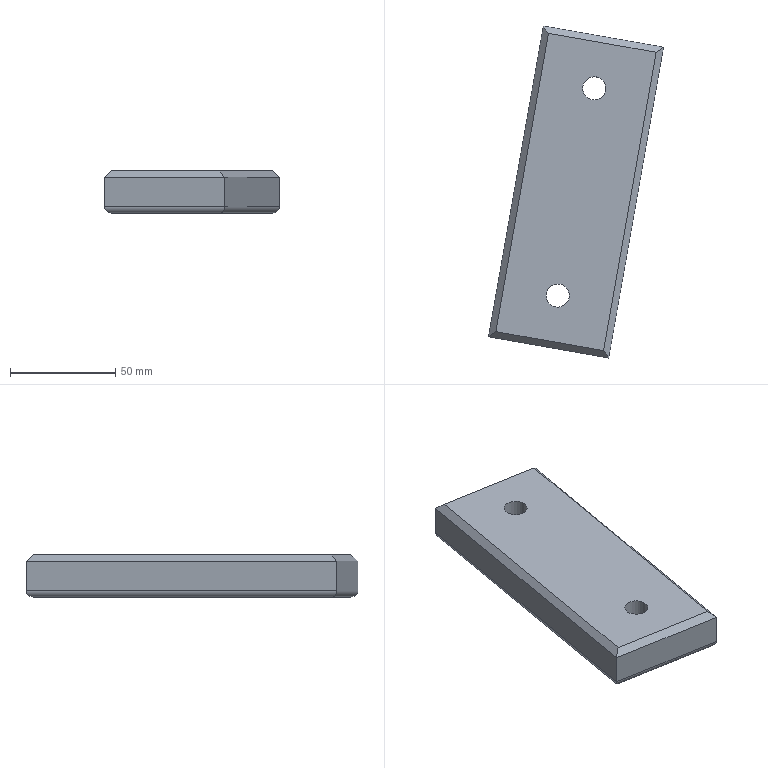Part | NX | features solid 2 | 1 solid | 20 faces | box 83.166 x 157.793 x 20 mm | volume 164078 mm3 | plane 12 | cylinder 8 | commonest cylinder face diameters 6 x4 11 x2 17.5 x2
STEP:
#1=CARTESIAN_POINT('',(863.455,-228.407,187.));
#2=VERTEX_POINT('',#1);
#3=CARTESIAN_POINT('',(863.455,-228.407,173.));
#4=VERTEX_POINT('',#3);
#5=CARTESIAN_POINT('',(863.455,-228.407,190.));
#6=DIRECTION('',(0.,0.,-1.));
#7=VECTOR('',#6,1000.);
#8=LINE('',#5,#7);
#9=EDGE_CURVE('',#2,#4,#8,.T.);
#10=ORIENTED_EDGE('',*,*,#9,.F.);
#11=CARTESIAN_POINT('',(806.336,-218.336,187.));
#12=VERTEX_POINT('',#11);
#13=CARTESIAN_POINT('',(806.336,-218.336,187.));
#14=DIRECTION('',(-0.9848,0.1736,0.));
#15=VECTOR('',#14,1000.);
#16=LINE('',#13,#15);
#17=EDGE_CURVE('',#2,#12,#16,.T.);
#18=ORIENTED_EDGE('',*,*,#17,.T.);
#19=CARTESIAN_POINT('',(806.336,-218.336,173.));
#20=VERTEX_POINT('',#19);
#21=CARTESIAN_POINT('',(806.336,-218.336,190.));
#22=DIRECTION('',(0.,0.,-1.));
#23=VECTOR('',#22,1000.);
#24=LINE('',#21,#23);
#25=EDGE_CURVE('',#12,#20,#24,.T.);
#26=ORIENTED_EDGE('',*,*,#25,.T.);
#27=CARTESIAN_POINT('',(806.336,-218.336,173.));
#28=DIRECTION('',(0.9848,-0.1736,0.));
#29=VECTOR('',#28,1000.);
#30=LINE('',#27,#29);
#31=EDGE_CURVE('',#20,#4,#30,.T.);
#32=ORIENTED_EDGE('',*,*,#31,.T.);
#33=EDGE_LOOP('',(#10,#18,#26,#32));
#34=FACE_BOUND('',#33,.T.);
#35=CARTESIAN_POINT('',(806.336,-218.336,190.));
#36=DIRECTION('',(0.1736,0.9848,0.));
#37=DIRECTION('',(0.,0.,-1.));
#38=AXIS2_PLACEMENT_3D('',#35,#36,#37);
#39=PLANE('',#38);
#40=ADVANCED_FACE('',(#34),#39,.F.);
#41=CARTESIAN_POINT('',(889.503,-80.686,187.));
#42=VERTEX_POINT('',#41);
#43=CARTESIAN_POINT('',(889.503,-80.686,173.));
#44=VERTEX_POINT('',#43);
#45=CARTESIAN_POINT('',(889.503,-80.686,190.));
#46=DIRECTION('',(0.,0.,-1.));
#47=VECTOR('',#46,1000.);
#48=LINE('',#45,#47);
#49=EDGE_CURVE('',#42,#44,#48,.T.);
#50=ORIENTED_EDGE('',*,*,#49,.F.);
#51=CARTESIAN_POINT('',(863.455,-228.407,187.));
#52=DIRECTION('',(-0.1736,-0.9848,0.));
#53=VECTOR('',#52,1000.);
#54=LINE('',#51,#53);
#55=EDGE_CURVE('',#42,#2,#54,.T.);
#56=ORIENTED_EDGE('',*,*,#55,.T.);
#57=ORIENTED_EDGE('',*,*,#9,.T.);
#58=CARTESIAN_POINT('',(863.455,-228.407,173.));
#59=DIRECTION('',(0.1736,0.9848,0.));
#60=VECTOR('',#59,1000.);
#61=LINE('',#58,#60);
#62=EDGE_CURVE('',#4,#44,#61,.T.);
#63=ORIENTED_EDGE('',*,*,#62,.T.);
#64=EDGE_LOOP('',(#50,#56,#57,#63));
#65=FACE_BOUND('',#64,.T.);
#66=CARTESIAN_POINT('',(863.455,-228.407,190.));
#67=DIRECTION('',(-0.9848,0.1736,0.));
#68=DIRECTION('',(0.,0.,1.));
#69=AXIS2_PLACEMENT_3D('',#66,#67,#68);
#70=PLANE('',#69);
#71=ADVANCED_FACE('',(#65),#70,.F.);
#72=CARTESIAN_POINT('',(832.384,-70.615,187.));
#73=VERTEX_POINT('',#72);
#74=CARTESIAN_POINT('',(832.384,-70.615,173.));
#75=VERTEX_POINT('',#74);
#76=CARTESIAN_POINT('',(832.384,-70.615,190.));
#77=DIRECTION('',(0.,0.,-1.));
#78=VECTOR('',#77,1000.);
#79=LINE('',#76,#78);
#80=EDGE_CURVE('',#73,#75,#79,.T.);
#81=ORIENTED_EDGE('',*,*,#80,.F.);
#82=CARTESIAN_POINT('',(889.503,-80.686,187.));
#83=DIRECTION('',(0.9848,-0.1736,0.));
#84=VECTOR('',#83,1000.);
#85=LINE('',#82,#84);
#86=EDGE_CURVE('',#73,#42,#85,.T.);
#87=ORIENTED_EDGE('',*,*,#86,.T.);
#88=ORIENTED_EDGE('',*,*,#49,.T.);
#89=CARTESIAN_POINT('',(889.503,-80.686,173.));
#90=DIRECTION('',(-0.9848,0.1736,0.));
#91=VECTOR('',#90,1000.);
#92=LINE('',#89,#91);
#93=EDGE_CURVE('',#44,#75,#92,.T.);
#94=ORIENTED_EDGE('',*,*,#93,.T.);
#95=EDGE_LOOP('',(#81,#87,#88,#94));
#96=FACE_BOUND('',#95,.T.);
#97=CARTESIAN_POINT('',(889.503,-80.686,190.));
#98=DIRECTION('',(-0.1736,-0.9848,0.));
#99=DIRECTION('',(0.,0.,1.));
#100=AXIS2_PLACEMENT_3D('',#97,#98,#99);
#101=PLANE('',#100);
#102=ADVANCED_FACE('',(#96),#101,.F.);
#103=ORIENTED_EDGE('',*,*,#25,.F.);
#104=CARTESIAN_POINT('',(832.384,-70.615,187.));
#105=DIRECTION('',(0.1736,0.9848,0.));
#106=VECTOR('',#105,1000.);
#107=LINE('',#104,#106);
#108=EDGE_CURVE('',#12,#73,#107,.T.);
#109=ORIENTED_EDGE('',*,*,#108,.T.);
#110=ORIENTED_EDGE('',*,*,#80,.T.);
#111=CARTESIAN_POINT('',(832.384,-70.615,173.));
#112=DIRECTION('',(-0.1736,-0.9848,0.));
#113=VECTOR('',#112,1000.);
#114=LINE('',#111,#113);
#115=EDGE_CURVE('',#75,#20,#114,.T.);
#116=ORIENTED_EDGE('',*,*,#115,.T.);
#117=EDGE_LOOP('',(#103,#109,#110,#116));
#118=FACE_BOUND('',#117,.T.);
#119=CARTESIAN_POINT('',(832.384,-70.615,190.));
#120=DIRECTION('',(0.9848,-0.1736,0.));
#121=DIRECTION('',(0.1736,0.9848,0.));
#122=AXIS2_PLACEMENT_3D('',#119,#120,#121);
#123=PLANE('',#122);
#124=ADVANCED_FACE('',(#118),#123,.F.);
#125=CARTESIAN_POINT('',(861.022,-224.932,190.));
#126=VERTEX_POINT('',#125);
#127=CARTESIAN_POINT('',(886.027,-83.12,190.));
#128=VERTEX_POINT('',#127);
#129=CARTESIAN_POINT('',(886.548,-80.165,190.));
#130=DIRECTION('',(0.1736,0.9848,0.));
#131=VECTOR('',#130,1000.);
#132=LINE('',#129,#131);
#133=EDGE_CURVE('',#126,#128,#132,.T.);
#134=ORIENTED_EDGE('',*,*,#133,.T.);
#135=CARTESIAN_POINT('',(834.817,-74.09,190.));
#136=VERTEX_POINT('',#135);
#137=CARTESIAN_POINT('',(831.863,-73.569,190.));
#138=DIRECTION('',(-0.9848,0.1736,0.));
#139=VECTOR('',#138,1000.);
#140=LINE('',#137,#139);
#141=EDGE_CURVE('',#128,#136,#140,.T.);
#142=ORIENTED_EDGE('',*,*,#141,.T.);
#143=CARTESIAN_POINT('',(809.812,-215.902,190.));
#144=VERTEX_POINT('',#143);
#145=CARTESIAN_POINT('',(809.291,-218.857,190.));
#146=DIRECTION('',(-0.1736,-0.9848,0.));
#147=VECTOR('',#146,1000.);
#148=LINE('',#145,#147);
#149=EDGE_CURVE('',#136,#144,#148,.T.);
#150=ORIENTED_EDGE('',*,*,#149,.T.);
#151=CARTESIAN_POINT('',(863.976,-225.453,190.));
#152=DIRECTION('',(0.9848,-0.1736,0.));
#153=VECTOR('',#152,1000.);
#154=LINE('',#151,#153);
#155=EDGE_CURVE('',#144,#126,#154,.T.);
#156=ORIENTED_EDGE('',*,*,#155,.T.);
#157=EDGE_LOOP('',(#134,#142,#150,#156));
#158=FACE_BOUND('',#157,.T.);
#159=CARTESIAN_POINT('',(857.557,-94.854,190.));
#160=VERTEX_POINT('',#159);
#161=CARTESIAN_POINT('',(856.602,-100.271,190.));
#162=DIRECTION('',(0.,0.,1.));
#163=DIRECTION('',(0.1736,0.9848,0.));
#164=AXIS2_PLACEMENT_3D('',#161,#162,#163);
#165=CIRCLE('',#164,5.5);
#166=EDGE_CURVE('',#160,#160,#165,.T.);
#167=ORIENTED_EDGE('',*,*,#166,.F.);
#168=EDGE_LOOP('',(#167));
#169=FACE_BOUND('',#168,.T.);
#170=CARTESIAN_POINT('',(840.192,-193.335,190.));
#171=VERTEX_POINT('',#170);
#172=CARTESIAN_POINT('',(839.237,-198.751,190.));
#173=DIRECTION('',(0.,0.,1.));
#174=DIRECTION('',(0.1736,0.9848,0.));
#175=AXIS2_PLACEMENT_3D('',#172,#173,#174);
#176=CIRCLE('',#175,5.5);
#177=EDGE_CURVE('',#171,#171,#176,.T.);
#178=ORIENTED_EDGE('',*,*,#177,.F.);
#179=EDGE_LOOP('',(#178));
#180=FACE_BOUND('',#179,.T.);
#181=CARTESIAN_POINT('',(863.455,-228.407,190.));
#182=DIRECTION('',(0.,0.,1.));
#183=DIRECTION('',(0.1736,0.9848,0.));
#184=AXIS2_PLACEMENT_3D('',#181,#182,#183);
#185=PLANE('',#184);
#186=ADVANCED_FACE('',(#158,#169,#180),#185,.T.);
#187=CARTESIAN_POINT('',(861.022,-224.932,170.));
#188=VERTEX_POINT('',#187);
#189=CARTESIAN_POINT('',(809.812,-215.902,170.));
#190=VERTEX_POINT('',#189);
#191=CARTESIAN_POINT('',(863.976,-225.453,170.));
#192=DIRECTION('',(0.9848,-0.1736,0.));
#193=VECTOR('',#192,1000.);
#194=LINE('',#191,#193);
#195=EDGE_CURVE('',#188,#190,#194,.F.);
#196=ORIENTED_EDGE('',*,*,#195,.T.);
#197=CARTESIAN_POINT('',(834.817,-74.09,170.));
#198=VERTEX_POINT('',#197);
#199=CARTESIAN_POINT('',(809.291,-218.857,170.));
#200=DIRECTION('',(-0.1736,-0.9848,0.));
#201=VECTOR('',#200,1000.);
#202=LINE('',#199,#201);
#203=EDGE_CURVE('',#190,#198,#202,.F.);
#204=ORIENTED_EDGE('',*,*,#203,.T.);
#205=CARTESIAN_POINT('',(886.027,-83.12,170.));
#206=VERTEX_POINT('',#205);
#207=CARTESIAN_POINT('',(888.982,-83.641,170.));
#208=DIRECTION('',(-0.9848,0.1736,0.));
#209=VECTOR('',#208,1000.);
#210=LINE('',#207,#209);
#211=EDGE_CURVE('',#198,#206,#210,.F.);
#212=ORIENTED_EDGE('',*,*,#211,.T.);
#213=CARTESIAN_POINT('',(860.501,-227.887,170.));
#214=DIRECTION('',(0.1736,0.9848,0.));
#215=VECTOR('',#214,1000.);
#216=LINE('',#213,#215);
#217=EDGE_CURVE('',#206,#188,#216,.F.);
#218=ORIENTED_EDGE('',*,*,#217,.T.);
#219=EDGE_LOOP('',(#196,#204,#212,#218));
#220=FACE_BOUND('',#219,.T.);
#221=CARTESIAN_POINT('',(858.121,-91.654,170.));
#222=VERTEX_POINT('',#221);
#223=CARTESIAN_POINT('',(856.602,-100.271,170.));
#224=DIRECTION('',(0.,0.,1.));
#225=DIRECTION('',(0.1736,0.9848,0.));
#226=AXIS2_PLACEMENT_3D('',#223,#224,#225);
#227=CIRCLE('',#226,8.75);
#228=EDGE_CURVE('',#222,#222,#227,.T.);
#229=ORIENTED_EDGE('',*,*,#228,.T.);
#230=EDGE_LOOP('',(#229));
#231=FACE_BOUND('',#230,.T.);
#232=CARTESIAN_POINT('',(840.756,-190.134,170.));
#233=VERTEX_POINT('',#232);
#234=CARTESIAN_POINT('',(839.237,-198.751,170.));
#235=DIRECTION('',(0.,0.,1.));
#236=DIRECTION('',(0.1736,0.9848,0.));
#237=AXIS2_PLACEMENT_3D('',#234,#235,#236);
#238=CIRCLE('',#237,8.75);
#239=EDGE_CURVE('',#233,#233,#238,.T.);
#240=ORIENTED_EDGE('',*,*,#239,.T.);
#241=EDGE_LOOP('',(#240));
#242=FACE_BOUND('',#241,.T.);
#243=CARTESIAN_POINT('',(863.455,-228.407,170.));
#244=DIRECTION('',(0.,0.,1.));
#245=DIRECTION('',(0.1736,0.9848,0.));
#246=AXIS2_PLACEMENT_3D('',#243,#244,#245);
#247=PLANE('',#246);
#248=ADVANCED_FACE('',(#220,#231,#242),#247,.F.);
#249=ORIENTED_EDGE('',*,*,#177,.T.);
#250=EDGE_LOOP('',(#249));
#251=FACE_BOUND('',#250,.T.);
#252=CARTESIAN_POINT('',(840.192,-193.335,182.));
#253=VERTEX_POINT('',#252);
#254=CARTESIAN_POINT('',(839.237,-198.751,182.));
#255=DIRECTION('',(0.,0.,1.));
#256=DIRECTION('',(0.1736,0.9848,0.));
#257=AXIS2_PLACEMENT_3D('',#254,#255,#256);
#258=CIRCLE('',#257,5.5);
#259=EDGE_CURVE('',#253,#253,#258,.T.);
#260=ORIENTED_EDGE('',*,*,#259,.F.);
#261=EDGE_LOOP('',(#260));
#262=FACE_BOUND('',#261,.T.);
#263=CARTESIAN_POINT('',(839.237,-198.751,220.));
#264=DIRECTION('',(0.,0.,1.));
#265=DIRECTION('',(0.1736,0.9848,0.));
#266=AXIS2_PLACEMENT_3D('',#263,#264,#265);
#267=CYLINDRICAL_SURFACE('',#266,5.5);
#268=ADVANCED_FACE('',(#251,#262),#267,.F.);
#269=ORIENTED_EDGE('',*,*,#259,.T.);
#270=EDGE_LOOP('',(#269));
#271=FACE_BOUND('',#270,.T.);
#272=CARTESIAN_POINT('',(840.756,-190.134,182.));
#273=VERTEX_POINT('',#272);
#274=CARTESIAN_POINT('',(839.237,-198.751,182.));
#275=DIRECTION('',(0.,0.,1.));
#276=DIRECTION('',(0.1736,0.9848,0.));
#277=AXIS2_PLACEMENT_3D('',#274,#275,#276);
#278=CIRCLE('',#277,8.75);
#279=EDGE_CURVE('',#273,#273,#278,.T.);
#280=ORIENTED_EDGE('',*,*,#279,.F.);
#281=EDGE_LOOP('',(#280));
#282=FACE_BOUND('',#281,.T.);
#283=CARTESIAN_POINT('',(839.237,-198.751,182.));
#284=DIRECTION('',(0.,0.,1.));
#285=DIRECTION('',(0.1736,0.9848,0.));
#286=AXIS2_PLACEMENT_3D('',#283,#284,#285);
#287=PLANE('',#286);
#288=ADVANCED_FACE('',(#271,#282),#287,.F.);
#289=ORIENTED_EDGE('',*,*,#279,.T.);
#290=EDGE_LOOP('',(#289));
#291=FACE_BOUND('',#290,.T.);
#292=ORIENTED_EDGE('',*,*,#239,.F.);
#293=EDGE_LOOP('',(#292));
#294=FACE_BOUND('',#293,.T.);
#295=CARTESIAN_POINT('',(839.237,-198.751,170.));
#296=DIRECTION('',(0.,0.,1.));
#297=DIRECTION('',(0.1736,0.9848,0.));
#298=AXIS2_PLACEMENT_3D('',#295,#296,#297);
#299=CYLINDRICAL_SURFACE('',#298,8.75);
#300=ADVANCED_FACE('',(#291,#294),#299,.F.);
#301=ORIENTED_EDGE('',*,*,#166,.T.);
#302=EDGE_LOOP('',(#301));
#303=FACE_BOUND('',#302,.T.);
#304=CARTESIAN_POINT('',(857.557,-94.854,182.));
#305=VERTEX_POINT('',#304);
#306=CARTESIAN_POINT('',(856.602,-100.271,182.));
#307=DIRECTION('',(0.,0.,1.));
#308=DIRECTION('',(0.1736,0.9848,0.));
#309=AXIS2_PLACEMENT_3D('',#306,#307,#308);
#310=CIRCLE('',#309,5.5);
#311=EDGE_CURVE('',#305,#305,#310,.T.);
#312=ORIENTED_EDGE('',*,*,#311,.F.);
#313=EDGE_LOOP('',(#312));
#314=FACE_BOUND('',#313,.T.);
#315=CARTESIAN_POINT('',(856.602,-100.271,220.));
#316=DIRECTION('',(0.,0.,1.));
#317=DIRECTION('',(0.1736,0.9848,0.));
#318=AXIS2_PLACEMENT_3D('',#315,#316,#317);
#319=CYLINDRICAL_SURFACE('',#318,5.5);
#320=ADVANCED_FACE('',(#303,#314),#319,.F.);
#321=ORIENTED_EDGE('',*,*,#311,.T.);
#322=EDGE_LOOP('',(#321));
#323=FACE_BOUND('',#322,.T.);
#324=CARTESIAN_POINT('',(858.121,-91.654,182.));
#325=VERTEX_POINT('',#324);
#326=CARTESIAN_POINT('',(856.602,-100.271,182.));
#327=DIRECTION('',(0.,0.,1.));
#328=DIRECTION('',(0.1736,0.9848,0.));
#329=AXIS2_PLACEMENT_3D('',#326,#327,#328);
#330=CIRCLE('',#329,8.75);
#331=EDGE_CURVE('',#325,#325,#330,.T.);
#332=ORIENTED_EDGE('',*,*,#331,.F.);
#333=EDGE_LOOP('',(#332));
#334=FACE_BOUND('',#333,.T.);
#335=CARTESIAN_POINT('',(856.602,-100.271,182.));
#336=DIRECTION('',(0.,0.,1.));
#337=DIRECTION('',(0.1736,0.9848,0.));
#338=AXIS2_PLACEMENT_3D('',#335,#336,#337);
#339=PLANE('',#338);
#340=ADVANCED_FACE('',(#323,#334),#339,.F.);
#341=ORIENTED_EDGE('',*,*,#331,.T.);
#342=EDGE_LOOP('',(#341));
#343=FACE_BOUND('',#342,.T.);
#344=ORIENTED_EDGE('',*,*,#228,.F.);
#345=EDGE_LOOP('',(#344));
#346=FACE_BOUND('',#345,.T.);
#347=CARTESIAN_POINT('',(856.602,-100.271,170.));
#348=DIRECTION('',(0.,0.,1.));
#349=DIRECTION('',(0.1736,0.9848,0.));
#350=AXIS2_PLACEMENT_3D('',#347,#348,#349);
#351=CYLINDRICAL_SURFACE('',#350,8.75);
#352=ADVANCED_FACE('',(#343,#346),#351,.F.);
#353=CARTESIAN_POINT('',(861.022,-224.932,173.));
#354=DIRECTION('',(0.8192,0.5736,0.));
#355=DIRECTION('',(0.5736,-0.8192,0.));
#356=AXIS2_PLACEMENT_3D('',#353,#354,#355);
#357=ELLIPSE('',#356,4.243,3.);
#358=EDGE_CURVE('',#188,#4,#357,.F.);
#359=ORIENTED_EDGE('',*,*,#358,.F.);
#360=ORIENTED_EDGE('',*,*,#217,.F.);
#361=CARTESIAN_POINT('',(886.027,-83.12,173.));
#362=DIRECTION('',(-0.5736,0.8192,0.));
#363=DIRECTION('',(0.8192,0.5736,0.));
#364=AXIS2_PLACEMENT_3D('',#361,#362,#363);
#365=ELLIPSE('',#364,4.243,3.);
#366=EDGE_CURVE('',#44,#206,#365,.T.);
#367=ORIENTED_EDGE('',*,*,#366,.F.);
#368=ORIENTED_EDGE('',*,*,#62,.F.);
#369=EDGE_LOOP('',(#359,#360,#367,#368));
#370=FACE_BOUND('',#369,.T.);
#371=CARTESIAN_POINT('',(860.501,-227.887,173.));
#372=DIRECTION('',(0.1736,0.9848,0.));
#373=DIRECTION('',(0.,0.,-1.));
#374=AXIS2_PLACEMENT_3D('',#371,#372,#373);
#375=CYLINDRICAL_SURFACE('',#374,3.);
#376=ADVANCED_FACE('',(#370),#375,.T.);
#377=ORIENTED_EDGE('',*,*,#366,.T.);
#378=ORIENTED_EDGE('',*,*,#211,.F.);
#379=CARTESIAN_POINT('',(834.817,-74.09,173.));
#380=DIRECTION('',(-0.8192,-0.5736,0.));
#381=DIRECTION('',(-0.5736,0.8192,0.));
#382=AXIS2_PLACEMENT_3D('',#379,#380,#381);
#383=ELLIPSE('',#382,4.243,3.);
#384=EDGE_CURVE('',#75,#198,#383,.T.);
#385=ORIENTED_EDGE('',*,*,#384,.F.);
#386=ORIENTED_EDGE('',*,*,#93,.F.);
#387=EDGE_LOOP('',(#377,#378,#385,#386));
#388=FACE_BOUND('',#387,.T.);
#389=CARTESIAN_POINT('',(888.982,-83.641,173.));
#390=DIRECTION('',(-0.9848,0.1736,0.));
#391=DIRECTION('',(0.,0.,1.));
#392=AXIS2_PLACEMENT_3D('',#389,#390,#391);
#393=CYLINDRICAL_SURFACE('',#392,3.);
#394=ADVANCED_FACE('',(#388),#393,.T.);
#395=ORIENTED_EDGE('',*,*,#358,.T.);
#396=ORIENTED_EDGE('',*,*,#31,.F.);
#397=CARTESIAN_POINT('',(809.812,-215.902,173.));
#398=DIRECTION('',(0.5736,-0.8192,0.));
#399=DIRECTION('',(0.8192,0.5736,0.));
#400=AXIS2_PLACEMENT_3D('',#397,#398,#399);
#401=ELLIPSE('',#400,4.243,3.);
#402=EDGE_CURVE('',#190,#20,#401,.F.);
#403=ORIENTED_EDGE('',*,*,#402,.F.);
#404=ORIENTED_EDGE('',*,*,#195,.F.);
#405=EDGE_LOOP('',(#395,#396,#403,#404));
#406=FACE_BOUND('',#405,.T.);
#407=CARTESIAN_POINT('',(806.857,-215.381,173.));
#408=DIRECTION('',(0.9848,-0.1736,0.));
#409=DIRECTION('',(0.,0.,-1.));
#410=AXIS2_PLACEMENT_3D('',#407,#408,#409);
#411=CYLINDRICAL_SURFACE('',#410,3.);
#412=ADVANCED_FACE('',(#406),#411,.T.);
#413=ORIENTED_EDGE('',*,*,#384,.T.);
#414=ORIENTED_EDGE('',*,*,#203,.F.);
#415=ORIENTED_EDGE('',*,*,#402,.T.);
#416=ORIENTED_EDGE('',*,*,#115,.F.);
#417=EDGE_LOOP('',(#413,#414,#415,#416));
#418=FACE_BOUND('',#417,.T.);
#419=CARTESIAN_POINT('',(835.338,-71.136,173.));
#420=DIRECTION('',(-0.1736,-0.9848,0.));
#421=DIRECTION('',(0.9848,-0.1736,0.));
#422=AXIS2_PLACEMENT_3D('',#419,#420,#421);
#423=CYLINDRICAL_SURFACE('',#422,3.);
#424=ADVANCED_FACE('',(#418),#423,.T.);
#425=CARTESIAN_POINT('',(808.653,-216.714,189.));
#426=DIRECTION('',(0.6688,0.4683,0.5774));
#427=VECTOR('',#426,1000.);
#428=LINE('',#425,#427);
#429=EDGE_CURVE('',#12,#144,#428,.T.);
#430=ORIENTED_EDGE('',*,*,#429,.F.);
#431=ORIENTED_EDGE('',*,*,#17,.F.);
#432=CARTESIAN_POINT('',(861.833,-226.091,189.));
#433=DIRECTION('',(-0.4683,0.6688,0.5774));
#434=VECTOR('',#433,1000.);
#435=LINE('',#432,#434);
#436=EDGE_CURVE('',#126,#2,#435,.F.);
#437=ORIENTED_EDGE('',*,*,#436,.F.);
#438=ORIENTED_EDGE('',*,*,#155,.F.);
#439=EDGE_LOOP('',(#430,#431,#437,#438));
#440=FACE_BOUND('',#439,.T.);
#441=CARTESIAN_POINT('',(863.976,-225.453,190.));
#442=DIRECTION('',(-0.1228,-0.6964,0.7071));
#443=DIRECTION('',(0.1228,0.6964,0.7071));
#444=AXIS2_PLACEMENT_3D('',#441,#442,#443);
#445=PLANE('',#444);
#446=ADVANCED_FACE('',(#440),#445,.T.);
#447=ORIENTED_EDGE('',*,*,#436,.T.);
#448=ORIENTED_EDGE('',*,*,#55,.F.);
#449=CARTESIAN_POINT('',(829.263,-122.867,239.));
#450=DIRECTION('',(-0.6688,-0.4683,0.5774));
#451=VECTOR('',#450,1000.);
#452=LINE('',#449,#451);
#453=EDGE_CURVE('',#128,#42,#452,.F.);
#454=ORIENTED_EDGE('',*,*,#453,.F.);
#455=ORIENTED_EDGE('',*,*,#133,.F.);
#456=EDGE_LOOP('',(#447,#448,#454,#455));
#457=FACE_BOUND('',#456,.T.);
#458=CARTESIAN_POINT('',(860.501,-227.887,190.));
#459=DIRECTION('',(0.6964,-0.1228,0.7071));
#460=DIRECTION('',(0.6964,-0.1228,-0.7071));
#461=AXIS2_PLACEMENT_3D('',#458,#459,#460);
#462=PLANE('',#461);
#463=ADVANCED_FACE('',(#457),#462,.T.);
#464=ORIENTED_EDGE('',*,*,#429,.T.);
#465=ORIENTED_EDGE('',*,*,#149,.F.);
#466=CARTESIAN_POINT('',(874.564,-130.854,239.));
#467=DIRECTION('',(-0.4683,0.6688,-0.5774));
#468=VECTOR('',#467,1000.);
#469=LINE('',#466,#468);
#470=EDGE_CURVE('',#73,#136,#469,.F.);
#471=ORIENTED_EDGE('',*,*,#470,.F.);
#472=ORIENTED_EDGE('',*,*,#108,.F.);
#473=EDGE_LOOP('',(#464,#465,#471,#472));
#474=FACE_BOUND('',#473,.T.);
#475=CARTESIAN_POINT('',(809.291,-218.857,190.));
#476=DIRECTION('',(-0.6964,0.1228,0.7071));
#477=DIRECTION('',(0.6964,-0.1228,0.7071));
#478=AXIS2_PLACEMENT_3D('',#475,#476,#477);
#479=PLANE('',#478);
#480=ADVANCED_FACE('',(#474),#479,.T.);
#481=ORIENTED_EDGE('',*,*,#453,.T.);
#482=ORIENTED_EDGE('',*,*,#86,.F.);
#483=ORIENTED_EDGE('',*,*,#470,.T.);
#484=ORIENTED_EDGE('',*,*,#141,.F.);
#485=EDGE_LOOP('',(#481,#482,#483,#484));
#486=FACE_BOUND('',#485,.T.);
#487=CARTESIAN_POINT('',(888.982,-83.641,190.));
#488=DIRECTION('',(0.1228,0.6964,0.7071));
#489=DIRECTION('',(0.1228,0.6964,-0.7071));
#490=AXIS2_PLACEMENT_3D('',#487,#488,#489);
#491=PLANE('',#490);
#492=ADVANCED_FACE('',(#486),#491,.T.);
#493=CLOSED_SHELL('',(#40,#71,#102,#124,#186,#248,#268,#288,#300,#320,#340,#352,#376,#394,#412,#424,#446,#463,#480,#492));
#494=MANIFOLD_SOLID_BREP('',#493);
#495=(LENGTH_UNIT()NAMED_UNIT(*)SI_UNIT(.MILLI.,.METRE.));
#496=UNCERTAINTY_MEASURE_WITH_UNIT(LENGTH_MEASURE(0.00001),#495,'','');
#497=(NAMED_UNIT(*)PLANE_ANGLE_UNIT()SI_UNIT($,.RADIAN.));
#498=(NAMED_UNIT(*)SI_UNIT($,.STERADIAN.)SOLID_ANGLE_UNIT());
#499=(GEOMETRIC_REPRESENTATION_CONTEXT(3)GLOBAL_UNCERTAINTY_ASSIGNED_CONTEXT((#496))GLOBAL_UNIT_ASSIGNED_CONTEXT((#495,#497,#498))REPRESENTATION_CONTEXT('',''));
#500=ADVANCED_BREP_SHAPE_REPRESENTATION('',(#494),#499);